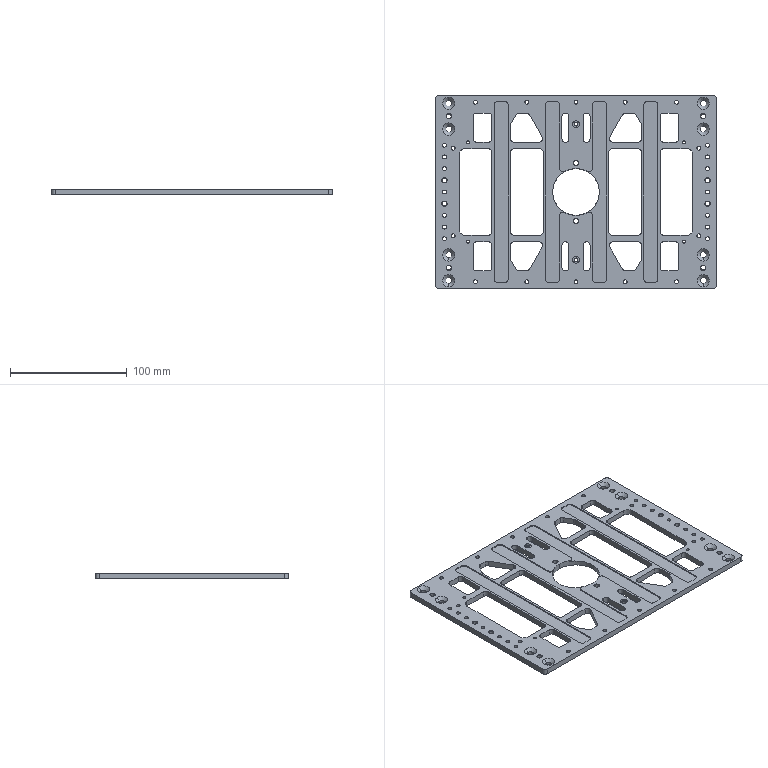NC program | NX | posted with a generic post | part box 240 x 165 x 5 mm
Lines 1 to 1758 of 12487:
N10 G17 G21 G94 G90
(DRILLING , TOOL : D6A45)
N12 T01 M6
N14 G54
N16 G17 G0 G90 X-42. Y-76.8 S5000 M3
N18 G43 Z30. H1
N20 G94 G81 G98 Z-1. F350. R3.
N22 X-86.
N24 X-108.75 Y-75.75
N26 Y-64.75
N28 Y-53.75
N30 X-92.502 Y-42.502
N32 X-105. Y-37.5
N34 X-112.5 Y-40.
N36 Y-30.
N38 Y-20.
N40 Y-10.
N42 Y0.
N44 Y10.
N46 Y20.
N48 Y30.
N50 Y40.
N52 X-105. Y37.5
N54 X-92.502 Y42.5
N56 X-108.75 Y53.75
N58 Y64.75
N60 Y75.75
N62 X-86. Y76.8
N64 X-42.
N66 X0.
N68 Y58.
N70 Y25.
N72 Y0.
N74 Y-25.
N76 Y-58.
N78 Y-76.8
N80 X42.
N82 X86.
N84 X108.75 Y-75.75
N86 Y-64.75
N88 Y-53.75
N90 X92.5 Y-42.502
N92 X105. Y-37.5
N94 X112.5 Y-40.
N96 Y-30.
N98 Y-20.
N100 Y-10.
N102 Y0.
N104 Y10.
N106 Y20.
N108 Y30.
N110 Y40.
N112 X105. Y37.5
N114 X92.5 Y42.5
N116 X108.75 Y53.75
N118 Y64.75
N120 Y75.75
N122 X86. Y76.8
N124 X42.
N126 G80
N128 G0 X42. Y76.8 Z30.
N130 M5
(DRILLING_COPY , TOOL : 3.3ZT)
N132 T03 M6
N134 G54
N136 G17 G0 G90 X-42. Y76.8 S2000 M3
N138 G43 Z30. H3
N140 G94 G83 G98 Z-7.491 F200. Q2. R3.
N142 X0.
N144 X42.
N146 X86.
N148 X105. Y37.5
N150 X112.5 Y40.
N152 Y30.
N154 Y20.
N156 Y0.
N158 Y-20.
N160 Y-30.
N162 Y-40.
N164 X105. Y-37.5
N166 X86. Y-76.8
N168 X42.
N170 X0.
N172 X-42.
N174 X-86.
N176 X-105. Y-37.5
N178 X-112.5 Y-40.
N180 Y-30.
N182 Y-20.
N184 Y0.
N186 Y20.
N188 Y30.
N190 Y40.
N192 X-105. Y37.5
N194 X-86. Y76.8
N196 G80
N198 G0 X-86. Y76.8 Z30.
N200 M5
(DRILLING_COPY_COPY_1 , TOOL : 3.2ZT)
N202 T16 M6
N204 G54
N206 G17 G0 G90 X0. Y58. S2000 M3
N208 G43 Z30. H16
N210 G94 G83 G98 Z-6.961 F200. Q2. R3.
N212 Y-58.
N214 G80
N216 G0 X0. Y-58. Z30.
N218 M5
(DRILLING_COPY_COPY , TOOL : 2.5ZT)
N220 T02 M6
N222 G54
N224 G17 G0 G90 X-92.502 Y42.5 S2000 M3
N226 G43 Z30. H2
N228 G94 G83 G98 Z-7.251 F150. Q2. R3.
N230 Y-42.502
N232 X92.5
N234 Y42.5
N236 G80
N238 G0 X92.5 Y42.5 Z30.
N240 M5
(DRILLING_COPY_COPY_1_COPY , TOOL : 3.8ZT)
N242 T18 M6
N244 G54
N246 G17 G0 G90 X-108.75 Y64.75 S2000 M3
N248 G43 Z30. H18
N250 G94 G83 G98 Z-7.142 F200. Q2. R3.
N252 X-112.5 Y10.
N254 Y-10.
N256 X-108.75 Y-64.75
N258 X0. Y-25.
N260 Y25.
N262 X108.75 Y64.75
N264 X112.5 Y10.
N266 Y-10.
N268 X108.75 Y-64.75
N270 G80
N272 G0 X108.75 Y-64.75 Z30.
N274 M5
(DRILLING_COPY_COPY_1_COPY_COPY , TOOL : 5.3ZT)
N276 T09 M6
N278 G54
N280 G17 G0 G90 X-108.75 Y-75.75 S2000 M3
N282 G43 Z30. H9
N284 G94 G83 G98 Z-7.592 F200. Q2. R3.
N286 Y-53.75
N288 Y53.75
N290 Y75.75
N292 X108.75
N294 Y53.75
N296 Y-53.75
N298 Y-75.75
N300 G80
N302 G0 X108.75 Y-75.75 Z30.
N304 M5
(ZLEVEL_PROFILE , TOOL : D10)
N306 T15 M6
N308 G54
N310 G17 G0 G90 X-45.413 Y87.6 S9500 M3
N312 G43 Z30. H15
N314 Z1.5
N316 G94 G1 X0. Z-0.88 F1000.
N318 X117. F3000.
N320 G2 X125.1 Y79.5 R8.1
N322 G1 Y-79.5
N324 G2 X117. Y-87.6 R8.1
N326 G1 X-117.
N328 G2 X-125.1 Y-79.5 R8.1
N330 G1 Y79.5
N332 G2 X-117. Y87.6 R8.1
N334 G1 X0.
N336 X117. Z-1.003
N338 X117.636 Y87.575 Z-1.004
N340 X118.267 Y87.5
N342 X118.891 Y87.376 Z-1.005
N344 X119.503 Y87.204 Z-1.006
N346 X120.1 Y86.983
N348 X120.677 Y86.717 Z-1.007
N350 X121.232 Y86.406 Z-1.008
N352 X121.761 Y86.053
N354 X122.261 Y85.659 Z-1.009
N356 X122.728 Y85.228 Z-1.01
N358 X123.159 Y84.761
N360 X123.553 Y84.261 Z-1.011
N362 X123.906 Y83.732 Z-1.012
N364 X124.217 Y83.177
N366 X124.483 Y82.6 Z-1.013
N368 X124.704 Y82.003 Z-1.014
N370 X124.876 Y81.391
N372 X125. Y80.767 Z-1.015
N374 X125.075 Y80.136 Z-1.016
N376 X125.1 Y79.5
N378 Y-79.5 Z-1.184
N380 X125.075 Y-80.136
N382 X125. Y-80.767 Z-1.185
N384 X124.876 Y-81.391 Z-1.186
N386 X124.704 Y-82.003
N388 X124.483 Y-82.6 Z-1.187
N390 X124.217 Y-83.177 Z-1.188
N392 X123.906 Y-83.732
N394 X123.553 Y-84.261 Z-1.189
N396 X123.159 Y-84.761 Z-1.19
N398 X122.728 Y-85.228
N400 X122.261 Y-85.659 Z-1.191
N402 X121.761 Y-86.053 Z-1.192
N404 X121.232 Y-86.406
N406 X120.677 Y-86.717 Z-1.193
N408 X120.1 Y-86.983 Z-1.194
N410 X119.503 Y-87.204
N412 X118.891 Y-87.376 Z-1.195
N414 X118.267 Y-87.5 Z-1.196
N416 X117.636 Y-87.575
N418 X117. Y-87.6 Z-1.197
N420 X-117. Z-1.443
N422 X-117.636 Y-87.575 Z-1.444
N424 X-118.267 Y-87.5
N426 X-118.891 Y-87.376 Z-1.445
N428 X-119.503 Y-87.204 Z-1.446
N430 X-120.1 Y-86.983
N432 X-120.677 Y-86.717 Z-1.447
N434 X-121.232 Y-86.406 Z-1.448
N436 X-121.761 Y-86.053
N438 X-122.261 Y-85.659 Z-1.449
N440 X-122.728 Y-85.228 Z-1.45
N442 X-123.159 Y-84.761
N444 X-123.553 Y-84.261 Z-1.451
N446 X-123.906 Y-83.732 Z-1.452
N448 X-124.217 Y-83.177
N450 X-124.483 Y-82.6 Z-1.453
N452 X-124.704 Y-82.003 Z-1.454
N454 X-124.876 Y-81.391
N456 X-125. Y-80.767 Z-1.455
N458 X-125.075 Y-80.136 Z-1.456
N460 X-125.1 Y-79.5
N462 Y79.5 Z-1.624
N464 X-125.075 Y80.136
N466 X-125. Y80.767 Z-1.625
N468 X-124.876 Y81.391 Z-1.626
N470 X-124.704 Y82.003
N472 X-124.483 Y82.6 Z-1.627
N474 X-124.217 Y83.177 Z-1.628
N476 X-123.906 Y83.732
N478 X-123.553 Y84.261 Z-1.629
N480 X-123.159 Y84.761 Z-1.63
N482 X-122.728 Y85.228
N484 X-122.261 Y85.659 Z-1.631
N486 X-121.761 Y86.053 Z-1.632
N488 X-121.232 Y86.406
N490 X-120.677 Y86.717 Z-1.633
N492 X-120.1 Y86.983 Z-1.634
N494 X-119.503 Y87.204
N496 X-118.891 Y87.376 Z-1.635
N498 X-118.267 Y87.5 Z-1.636
N500 X-117.636 Y87.575
N502 X-117. Y87.6 Z-1.637
N504 X0. Z-1.76
N506 X117. Z-1.883
N508 X117.636 Y87.575 Z-1.884
N510 X118.267 Y87.5
N512 X118.891 Y87.376 Z-1.885
N514 X119.503 Y87.204 Z-1.886
N516 X120.1 Y86.983
N518 X120.677 Y86.717 Z-1.887
N520 X121.232 Y86.406 Z-1.888
N522 X121.761 Y86.053
N524 X122.261 Y85.659 Z-1.889
N526 X122.728 Y85.228 Z-1.89
N528 X123.159 Y84.761
N530 X123.553 Y84.261 Z-1.891
N532 X123.906 Y83.732 Z-1.892
N534 X124.217 Y83.177
N536 X124.483 Y82.6 Z-1.893
N538 X124.704 Y82.003 Z-1.894
N540 X124.876 Y81.391
N542 X125. Y80.767 Z-1.895
N544 X125.075 Y80.136 Z-1.896
N546 X125.1 Y79.5
N548 Y-79.5 Z-2.064
N550 X125.075 Y-80.136
N552 X125. Y-80.767 Z-2.065
N554 X124.876 Y-81.391 Z-2.066
N556 X124.704 Y-82.003
N558 X124.483 Y-82.6 Z-2.067
N560 X124.217 Y-83.177 Z-2.068
N562 X123.906 Y-83.732
N564 X123.553 Y-84.261 Z-2.069
N566 X123.159 Y-84.761 Z-2.07
N568 X122.728 Y-85.228
N570 X122.261 Y-85.659 Z-2.071
N572 X121.761 Y-86.053 Z-2.072
N574 X121.232 Y-86.406
N576 X120.677 Y-86.717 Z-2.073
N578 X120.1 Y-86.983 Z-2.074
N580 X119.503 Y-87.204
N582 X118.891 Y-87.376 Z-2.075
N584 X118.267 Y-87.5 Z-2.076
N586 X117.636 Y-87.575
N588 X117. Y-87.6 Z-2.077
N590 X-117. Z-2.323
N592 X-117.636 Y-87.575 Z-2.324
N594 X-118.267 Y-87.5
N596 X-118.891 Y-87.376 Z-2.325
N598 X-119.503 Y-87.204 Z-2.326
N600 X-120.1 Y-86.983
N602 X-120.677 Y-86.717 Z-2.327
N604 X-121.232 Y-86.406 Z-2.328
N606 X-121.761 Y-86.053
N608 X-122.261 Y-85.659 Z-2.329
N610 X-122.728 Y-85.228 Z-2.33
N612 X-123.159 Y-84.761
N614 X-123.553 Y-84.261 Z-2.331
N616 X-123.906 Y-83.732 Z-2.332
N618 X-124.217 Y-83.177
N620 X-124.483 Y-82.6 Z-2.333
N622 X-124.704 Y-82.003 Z-2.334
N624 X-124.876 Y-81.391
N626 X-125. Y-80.767 Z-2.335
N628 X-125.075 Y-80.136 Z-2.336
N630 X-125.1 Y-79.5
N632 Y79.5 Z-2.504
N634 X-125.075 Y80.136
N636 X-125. Y80.767 Z-2.505
N638 X-124.876 Y81.391 Z-2.506
N640 X-124.704 Y82.003
N642 X-124.483 Y82.6 Z-2.507
N644 X-124.217 Y83.177 Z-2.508
N646 X-123.906 Y83.732
N648 X-123.553 Y84.261 Z-2.509
N650 X-123.159 Y84.761 Z-2.51
N652 X-122.728 Y85.228
N654 X-122.261 Y85.659 Z-2.511
N656 X-121.761 Y86.053 Z-2.512
N658 X-121.232 Y86.406
N660 X-120.677 Y86.717 Z-2.513
N662 X-120.1 Y86.983 Z-2.514
N664 X-119.503 Y87.204
N666 X-118.891 Y87.376 Z-2.515
N668 X-118.267 Y87.5 Z-2.516
N670 X-117.636 Y87.575
N672 X-117. Y87.6 Z-2.517
N674 X0. Z-2.64
N676 X117. Z-2.763
N678 X117.636 Y87.575 Z-2.764
N680 X118.267 Y87.5
N682 X118.891 Y87.376 Z-2.765
N684 X119.503 Y87.204 Z-2.766
N686 X120.1 Y86.983
N688 X120.677 Y86.717 Z-2.767
N690 X121.232 Y86.406 Z-2.768
N692 X121.761 Y86.053
N694 X122.261 Y85.659 Z-2.769
N696 X122.728 Y85.228 Z-2.77
N698 X123.159 Y84.761
N700 X123.553 Y84.261 Z-2.771
N702 X123.906 Y83.732 Z-2.772
N704 X124.217 Y83.177
N706 X124.483 Y82.6 Z-2.773
N708 X124.704 Y82.003 Z-2.774
N710 X124.876 Y81.391
N712 X125. Y80.767 Z-2.775
N714 X125.075 Y80.136 Z-2.776
N716 X125.1 Y79.5
N718 Y-79.5 Z-2.944
N720 X125.075 Y-80.136
N722 X125. Y-80.767 Z-2.945
N724 X124.876 Y-81.391 Z-2.946
N726 X124.704 Y-82.003
N728 X124.483 Y-82.6 Z-2.947
N730 X124.217 Y-83.177 Z-2.948
N732 X123.906 Y-83.732
N734 X123.553 Y-84.261 Z-2.949
N736 X123.159 Y-84.761 Z-2.95
N738 X122.728 Y-85.228
N740 X122.261 Y-85.659 Z-2.951
N742 X121.761 Y-86.053 Z-2.952
N744 X121.232 Y-86.406
N746 X120.677 Y-86.717 Z-2.953
N748 X120.1 Y-86.983 Z-2.954
N750 X119.503 Y-87.204
N752 X118.891 Y-87.376 Z-2.955
N754 X118.267 Y-87.5 Z-2.956
N756 X117.636 Y-87.575
N758 X117. Y-87.6 Z-2.957
N760 X-117. Z-3.203
N762 X-117.636 Y-87.575 Z-3.204
N764 X-118.267 Y-87.5
N766 X-118.891 Y-87.376 Z-3.205
N768 X-119.503 Y-87.204 Z-3.206
N770 X-120.1 Y-86.983
N772 X-120.677 Y-86.717 Z-3.207
N774 X-121.232 Y-86.406 Z-3.208
N776 X-121.761 Y-86.053
N778 X-122.261 Y-85.659 Z-3.209
N780 X-122.728 Y-85.228 Z-3.21
N782 X-123.159 Y-84.761
N784 X-123.553 Y-84.261 Z-3.211
N786 X-123.906 Y-83.732 Z-3.212
N788 X-124.217 Y-83.177
N790 X-124.483 Y-82.6 Z-3.213
N792 X-124.704 Y-82.003 Z-3.214
N794 X-124.876 Y-81.391
N796 X-125. Y-80.767 Z-3.215
N798 X-125.075 Y-80.136 Z-3.216
N800 X-125.1 Y-79.5
N802 Y79.5 Z-3.384
N804 X-125.075 Y80.136
N806 X-125. Y80.767 Z-3.385
N808 X-124.876 Y81.391 Z-3.386
N810 X-124.704 Y82.003
N812 X-124.483 Y82.6 Z-3.387
N814 X-124.217 Y83.177 Z-3.388
N816 X-123.906 Y83.732
N818 X-123.553 Y84.261 Z-3.389
N820 X-123.159 Y84.761 Z-3.39
N822 X-122.728 Y85.228
N824 X-122.261 Y85.659 Z-3.391
N826 X-121.761 Y86.053 Z-3.392
N828 X-121.232 Y86.406
N830 X-120.677 Y86.717 Z-3.393
N832 X-120.1 Y86.983 Z-3.394
N834 X-119.503 Y87.204
N836 X-118.891 Y87.376 Z-3.395
N838 X-118.267 Y87.5 Z-3.396
N840 X-117.636 Y87.575
N842 X-117. Y87.6 Z-3.397
N844 X0. Z-3.52
N846 X117. Z-3.643
N848 X117.636 Y87.575 Z-3.644
N850 X118.267 Y87.5
N852 X118.891 Y87.376 Z-3.645
N854 X119.503 Y87.204 Z-3.646
N856 X120.1 Y86.983
N858 X120.677 Y86.717 Z-3.647
N860 X121.232 Y86.406 Z-3.648
N862 X121.761 Y86.053
N864 X122.261 Y85.659 Z-3.649
N866 X122.728 Y85.228 Z-3.65
N868 X123.159 Y84.761
N870 X123.553 Y84.261 Z-3.651
N872 X123.906 Y83.732 Z-3.652
N874 X124.217 Y83.177
N876 X124.483 Y82.6 Z-3.653
N878 X124.704 Y82.003 Z-3.654
N880 X124.876 Y81.391
N882 X125. Y80.767 Z-3.655
N884 X125.075 Y80.136 Z-3.656
N886 X125.1 Y79.5
N888 Y-79.5 Z-3.824
N890 X125.075 Y-80.136
N892 X125. Y-80.767 Z-3.825
N894 X124.876 Y-81.391 Z-3.826
N896 X124.704 Y-82.003
N898 X124.483 Y-82.6 Z-3.827
N900 X124.217 Y-83.177 Z-3.828
N902 X123.906 Y-83.732
N904 X123.553 Y-84.261 Z-3.829
N906 X123.159 Y-84.761 Z-3.83
N908 X122.728 Y-85.228
N910 X122.261 Y-85.659 Z-3.831
N912 X121.761 Y-86.053 Z-3.832
N914 X121.232 Y-86.406
N916 X120.677 Y-86.717 Z-3.833
N918 X120.1 Y-86.983 Z-3.834
N920 X119.503 Y-87.204
N922 X118.891 Y-87.376 Z-3.835
N924 X118.267 Y-87.5 Z-3.836
N926 X117.636 Y-87.575
N928 X117. Y-87.6 Z-3.837
N930 X-117. Z-4.083
N932 X-117.636 Y-87.575 Z-4.084
N934 X-118.267 Y-87.5
N936 X-118.891 Y-87.376 Z-4.085
N938 X-119.503 Y-87.204 Z-4.086
N940 X-120.1 Y-86.983
N942 X-120.677 Y-86.717 Z-4.087
N944 X-121.232 Y-86.406 Z-4.088
N946 X-121.761 Y-86.053
N948 X-122.261 Y-85.659 Z-4.089
N950 X-122.728 Y-85.228 Z-4.09
N952 X-123.159 Y-84.761
N954 X-123.553 Y-84.261 Z-4.091
N956 X-123.906 Y-83.732 Z-4.092
N958 X-124.217 Y-83.177
N960 X-124.483 Y-82.6 Z-4.093
N962 X-124.704 Y-82.003 Z-4.094
N964 X-124.876 Y-81.391
N966 X-125. Y-80.767 Z-4.095
N968 X-125.075 Y-80.136 Z-4.096
N970 X-125.1 Y-79.5
N972 Y79.5 Z-4.264
N974 X-125.075 Y80.136
N976 X-125. Y80.767 Z-4.265
N978 X-124.876 Y81.391 Z-4.266
N980 X-124.704 Y82.003
N982 X-124.483 Y82.6 Z-4.267
N984 X-124.217 Y83.177 Z-4.268
N986 X-123.906 Y83.732
N988 X-123.553 Y84.261 Z-4.269
N990 X-123.159 Y84.761 Z-4.27
N992 X-122.728 Y85.228
N994 X-122.261 Y85.659 Z-4.271
N996 X-121.761 Y86.053 Z-4.272
N998 X-121.232 Y86.406
N1000 X-120.677 Y86.717 Z-4.273
N1002 X-120.1 Y86.983 Z-4.274
N1004 X-119.503 Y87.204
N1006 X-118.891 Y87.376 Z-4.275
N1008 X-118.267 Y87.5 Z-4.276
N1010 X-117.636 Y87.575
N1012 X-117. Y87.6 Z-4.277
N1014 X0. Z-4.4
N1016 X117.
N1018 G2 X125.1 Y79.5 R8.1
N1020 G1 Y-79.5
N1022 G2 X117. Y-87.6 R8.1
N1024 G1 X-117.
N1026 G2 X-125.1 Y-79.5 R8.1
N1028 G1 Y79.5
N1030 G2 X-117. Y87.6 R8.1
N1032 G1 X0.
N1034 Z-2.9
N1036 G0 Z30.
(ZLEVEL_PROFILE_COPY , TOOL : D10)
N1038 X77.1 Y61.503
N1040 Z1.5
N1042 G1 Y47.6 Z0.771 F1000.
N1044 X82.9 Z0.467
N1046 Y62.4 Z-0.308
N1048 X77.1 Z-0.612
N1050 Y55. Z-1.
N1052 Y47.6 F3000.
N1054 X82.9
N1056 Y62.4
N1058 X77.1
N1060 Y55.
N1062 Y47.6 Z-1.18
N1064 X82.9 Z-1.32
N1066 Y62.4 Z-1.68
N1068 X77.1 Z-1.82
N1070 Y55. Z-2.
N1072 Y47.6 Z-2.18
N1074 X82.9 Z-2.32
N1076 Y62.4 Z-2.68
N1078 X77.1 Z-2.82
N1080 Y55. Z-3.
N1082 Y47.6 Z-3.18
N1084 X82.9 Z-3.32
N1086 Y62.4 Z-3.68
N1088 X77.1 Z-3.82
N1090 Y55. Z-4.
N1092 Y47.6 Z-4.18
N1094 X82.9 Z-4.32
N1096 Y62.4 Z-4.68
N1098 X77.1 Z-4.82
N1100 Y55. Z-5.
N1102 Y47.6
N1104 X82.9
N1106 Y62.4
N1108 X77.1
N1110 Y55.
N1112 Z-3.5
N1114 G0 Z53.
N1116 X-41.675 Y58.887
N1118 Z1.5
N1120 G1 X-43.703 Y62.4 Z1.287 F1000.
N1122 X-47.297 Z1.099
N1124 X-50.9 Y56.16 Z0.721
N1126 Y47.6 Z0.273
N1128 X-35.158 Z-0.552
N1130 X-39.43 Y55. Z-1.
N1132 X-43.703 Y62.4 F3000.
N1134 X-47.297
N1136 X-50.9 Y56.16
N1138 Y47.6
N1140 X-35.158
N1142 X-39.43 Y55.
N1144 X-43.703 Y62.4 Z-1.164
N1146 X-47.297 Z-1.233
N1148 X-50.9 Y56.16 Z-1.371
N1150 Y47.6 Z-1.535
N1152 X-35.158 Z-1.836
N1154 X-39.43 Y55. Z-2.
N1156 X-43.703 Y62.4 Z-2.164
N1158 X-47.297 Z-2.233
N1160 X-50.9 Y56.16 Z-2.371
N1162 Y47.6 Z-2.535
N1164 X-35.158 Z-2.836
N1166 X-39.43 Y55. Z-3.
N1168 X-43.703 Y62.4 Z-3.164
N1170 X-47.297 Z-3.233
N1172 X-50.9 Y56.16 Z-3.371
N1174 Y47.6 Z-3.535
N1176 X-35.158 Z-3.836
N1178 X-39.43 Y55. Z-4.
N1180 X-43.703 Y62.4 Z-4.164
N1182 X-47.297 Z-4.233
N1184 X-50.9 Y56.16 Z-4.371
N1186 Y47.6 Z-4.535
N1188 X-35.158 Z-4.836
N1190 X-39.43 Y55. Z-5.
N1192 X-43.703 Y62.4
N1194 X-47.297
N1196 X-50.9 Y56.16
N1198 Y47.6
N1200 X-35.158
N1202 X-39.43 Y55.
N1204 Z-3.5
N1206 G0 Z53.
N1208 X77.1 Y-48.497
N1210 Z1.5
N1212 G1 Y-62.4 Z0.771 F1000.
N1214 X82.9 Z0.467
N1216 Y-47.6 Z-0.308
N1218 X77.1 Z-0.612
N1220 Y-55. Z-1.
N1222 Y-62.4 F3000.
N1224 X82.9
N1226 Y-47.6
N1228 X77.1
N1230 Y-55.
N1232 Y-62.4 Z-1.18
N1234 X82.9 Z-1.32
N1236 Y-47.6 Z-1.68
N1238 X77.1 Z-1.82
N1240 Y-55. Z-2.
N1242 Y-62.4 Z-2.18
N1244 X82.9 Z-2.32
N1246 Y-47.6 Z-2.68
N1248 X77.1 Z-2.82
N1250 Y-55. Z-3.
N1252 Y-62.4 Z-3.18
N1254 X82.9 Z-3.32
N1256 Y-47.6 Z-3.68
N1258 X77.1 Z-3.82
N1260 Y-55. Z-4.
N1262 Y-62.4 Z-4.18
N1264 X82.9 Z-4.32
N1266 Y-47.6 Z-4.68
N1268 X77.1 Z-4.82
N1270 Y-55. Z-5.
N1272 Y-62.4
N1274 X82.9
N1276 Y-47.6
N1278 X77.1
N1280 Y-55.
N1282 Z-3.5
N1284 G0 Z53.
N1286 X50.9 Y-50.994
N1288 Z1.5
N1290 G1 Y-47.6 Z1.322 F1000.
N1292 X35.158 Z0.497
N1294 X43.703 Y-62.4 Z-0.399
N1296 X47.297 Z-0.587
N1298 X50.9 Y-56.16 Z-0.965
N1300 Y-55.483 Z-1.
N1302 Y-47.6 F3000.
N1304 X35.158
N1306 X43.703 Y-62.4
N1308 X47.297
N1310 X50.9 Y-56.16
N1312 Y-55.483
N1314 Y-47.6 Z-1.151
N1316 X35.158 Z-1.453
N1318 X43.703 Y-62.4 Z-1.78
N1320 X47.297 Z-1.849
N1322 X50.9 Y-56.16 Z-1.987
N1324 Y-55.483 Z-2.
N1326 Y-47.6 Z-2.151
N1328 X35.158 Z-2.453
N1330 X43.703 Y-62.4 Z-2.78
N1332 X47.297 Z-2.849
N1334 X50.9 Y-56.16 Z-2.987
N1336 Y-55.483 Z-3.
N1338 Y-47.6 Z-3.151
N1340 X35.158 Z-3.453
N1342 X43.703 Y-62.4 Z-3.78
N1344 X47.297 Z-3.849
N1346 X50.9 Y-56.16 Z-3.987
N1348 Y-55.483 Z-4.
N1350 Y-47.6 Z-4.151
N1352 X35.158 Z-4.453
N1354 X43.703 Y-62.4 Z-4.78
N1356 X47.297 Z-4.849
N1358 X50.9 Y-56.16 Z-4.987
N1360 Y-55.483 Z-5.
N1362 Y-47.6
N1364 X35.158
N1366 X43.703 Y-62.4
N1368 X47.297
N1370 X50.9 Y-56.16
N1372 Y-55.483
N1374 Z-3.5
N1376 G0 Z53.
N1378 X-37.186 Y-51.113
N1380 Z1.5
N1382 G1 X-35.158 Y-47.6 Z1.287 F1000.
N1384 X-50.9 Z0.462
N1386 Y-56.16 Z0.014
N1388 X-47.297 Y-62.4 Z-0.364
N1390 X-43.703 Z-0.552
N1392 X-39.43 Y-55. Z-1.
N1394 X-35.158 Y-47.6 F3000.
N1396 X-50.9
N1398 Y-56.16
N1400 X-47.297 Y-62.4
N1402 X-43.703
N1404 X-39.43 Y-55.
N1406 X-35.158 Y-47.6 Z-1.164
N1408 X-50.9 Z-1.465
N1410 Y-56.16 Z-1.629
N1412 X-47.297 Y-62.4 Z-1.767
N1414 X-43.703 Z-1.836
N1416 X-39.43 Y-55. Z-2.
N1418 X-35.158 Y-47.6 Z-2.164
N1420 X-50.9 Z-2.465
N1422 Y-56.16 Z-2.629
N1424 X-47.297 Y-62.4 Z-2.767
N1426 X-43.703 Z-2.836
N1428 X-39.43 Y-55. Z-3.
N1430 X-35.158 Y-47.6 Z-3.164
N1432 X-50.9 Z-3.465
N1434 Y-56.16 Z-3.629
N1436 X-47.297 Y-62.4 Z-3.767
N1438 X-43.703 Z-3.836
N1440 X-39.43 Y-55. Z-4.
N1442 X-35.158 Y-47.6 Z-4.164
N1444 X-50.9 Z-4.465
N1446 Y-56.16 Z-4.629
N1448 X-47.297 Y-62.4 Z-4.767
N1450 X-43.703 Z-4.836
N1452 X-39.43 Y-55. Z-5.
N1454 X-35.158 Y-47.6
N1456 X-50.9
N1458 Y-56.16
N1460 X-47.297 Y-62.4
N1462 X-43.703
N1464 X-39.43 Y-55.
N1466 Z-3.5
N1468 G0 Z53.
N1470 X37.186 Y51.113
N1472 Z1.5
N1474 G1 X35.158 Y47.6 Z1.287 F1000.
N1476 X50.9 Z0.462
N1478 Y56.16 Z0.014
N1480 X47.297 Y62.4 Z-0.364
N1482 X43.703 Z-0.552
N1484 X39.43 Y55. Z-1.
N1486 X35.158 Y47.6 F3000.
N1488 X50.9
N1490 Y56.16
N1492 X47.297 Y62.4
N1494 X43.703
N1496 X39.43 Y55.
N1498 X35.158 Y47.6 Z-1.164
N1500 X50.9 Z-1.465
N1502 Y56.16 Z-1.629
N1504 X47.297 Y62.4 Z-1.767
N1506 X43.703 Z-1.836
N1508 X39.43 Y55. Z-2.
N1510 X35.158 Y47.6 Z-2.164
N1512 X50.9 Z-2.465
N1514 Y56.16 Z-2.629
N1516 X47.297 Y62.4 Z-2.767
N1518 X43.703 Z-2.836
N1520 X39.43 Y55. Z-3.
N1522 X35.158 Y47.6 Z-3.164
N1524 X50.9 Z-3.465
N1526 Y56.16 Z-3.629
N1528 X47.297 Y62.4 Z-3.767
N1530 X43.703 Z-3.836
N1532 X39.43 Y55. Z-4.
N1534 X35.158 Y47.6 Z-4.164
N1536 X50.9 Z-4.465
N1538 Y56.16 Z-4.629
N1540 X47.297 Y62.4 Z-4.767
N1542 X43.703 Z-4.836
N1544 X39.43 Y55. Z-5.
N1546 X35.158 Y47.6
N1548 X50.9
N1550 Y56.16
N1552 X47.297 Y62.4
N1554 X43.703
N1556 X39.43 Y55.
N1558 Z-3.5
N1560 G0 Z53.
N1562 X-77.1 Y-61.503
N1564 Z1.5
N1566 G1 Y-47.6 Z0.771 F1000.
N1568 X-82.9 Z0.467
N1570 Y-62.4 Z-0.308
N1572 X-77.1 Z-0.612
N1574 Y-55. Z-1.
N1576 Y-47.6 F3000.
N1578 X-82.9
N1580 Y-62.4
N1582 X-77.1
N1584 Y-55.
N1586 Y-47.6 Z-1.18
N1588 X-82.9 Z-1.32
N1590 Y-62.4 Z-1.68
N1592 X-77.1 Z-1.82
N1594 Y-55. Z-2.
N1596 Y-47.6 Z-2.18
N1598 X-82.9 Z-2.32
N1600 Y-62.4 Z-2.68
N1602 X-77.1 Z-2.82
N1604 Y-55. Z-3.
N1606 Y-47.6 Z-3.18
N1608 X-82.9 Z-3.32
N1610 Y-62.4 Z-3.68
N1612 X-77.1 Z-3.82
N1614 Y-55. Z-4.
N1616 Y-47.6 Z-4.18
N1618 X-82.9 Z-4.32
N1620 Y-62.4 Z-4.68
N1622 X-77.1 Z-4.82
N1624 Y-55. Z-5.
N1626 Y-47.6
N1628 X-82.9
N1630 Y-62.4
N1632 X-77.1
N1634 Y-55.
N1636 Z-3.5
N1638 G0 Z53.
N1640 Y48.497
N1642 Z1.5
N1644 G1 Y62.4 Z0.771 F1000.
N1646 X-82.9 Z0.467
N1648 Y47.6 Z-0.308
N1650 X-77.1 Z-0.612
N1652 Y55. Z-1.
N1654 Y62.4 F3000.
N1656 X-82.9
N1658 Y47.6
N1660 X-77.1
N1662 Y55.
N1664 Y62.4 Z-1.18
N1666 X-82.9 Z-1.32
N1668 Y47.6 Z-1.68
N1670 X-77.1 Z-1.82
N1672 Y55. Z-2.
N1674 Y62.4 Z-2.18
N1676 X-82.9 Z-2.32
N1678 Y47.6 Z-2.68
N1680 X-77.1 Z-2.82
N1682 Y55. Z-3.
N1684 Y62.4 Z-3.18
N1686 X-82.9 Z-3.32
N1688 Y47.6 Z-3.68
N1690 X-77.1 Z-3.82
N1692 Y55. Z-4.
N1694 Y62.4 Z-4.18
N1696 X-82.9 Z-4.32
N1698 Y47.6 Z-4.68
N1700 X-77.1 Z-4.82
N1702 Y55. Z-5.
N1704 Y62.4
N1706 X-82.9
N1708 Y47.6
N1710 X-77.1
N1712 Y55.
N1714 Z-3.5
N1716 G0 Z30.
(PLANAR_MILL , TOOL : D10)
N1718 X-84.1 Y5.897
N1720 Z1.5
N1722 G1 Y24.9 Z0.504
N1724 X-87.9 Z0.305
N1726 Y0. Z-1.
N1728 Y-24.9
N1730 X-84.1
N1732 Y24.9
N1734 X-87.9
N1736 Y0.
N1738 X-94.9
N1740 Y-31.9
N1742 X-77.1
N1744 Y31.9
N1746 X-94.9
N1748 Y0.
N1750 Z0.5
N1752 G0 X-84.1 Y5.897
N1754 G1 Y24.9 Z-0.496
N1756 X-87.9 Z-0.695
N1758 Y0. Z-2.
N1760 Y-24.9
N1762 X-84.1
N1764 Y24.9
N1766 X-87.9
N1768 Y0.
N1770 X-94.9
N1772 Y-31.9
N1774 X-77.1
N1776 Y31.9
N1778 X-94.9
N1780 Y0.
N1782 Z-0.5
N1784 G0 X-84.1 Y5.897
N1786 G1 Y24.9 Z-1.496
N1788 X-87.9 Z-1.695
N1790 Y0. Z-3.
N1792 Y-24.9
N1794 X-84.1
N1796 Y24.9
N1798 X-87.9
N1800 Y0.
N1802 X-94.9
N1804 Y-31.9
N1806 X-77.1
N1808 Y31.9
N1810 X-94.9
N1812 Y0.
N1814 Z-1.5
N1816 G0 X-84.1 Y5.897
N1818 G1 Y24.9 Z-2.496
N1820 X-87.9 Z-2.695
N1822 Y0. Z-4.
N1824 Y-24.9
N1826 X-84.1
N1828 Y24.9
N1830 X-87.9
N1832 Y0.
N1834 X-94.9
N1836 Y-31.9
N1838 X-77.1
N1840 Y31.9
N1842 X-94.9
N1844 Y0.
N1846 Z-2.5
N1848 G0 X-84.1 Y5.897
N1850 G1 Y24.9 Z-3.496
N1852 X-87.9 Z-3.695
N1854 Y0. Z-5.
N1856 Y-24.9
N1858 X-84.1
N1860 Y24.9
N1862 X-87.9
N1864 Y0.
N1866 X-94.9
N1868 Y-31.9
N1870 X-77.1
N1872 Y31.9
N1874 X-94.9
N1876 Y0.
N1878 Z-3.5
N1880 G0 Z30.
N1882 X-40.1 Y5.897
N1884 Z1.5
N1886 G1 Y24.9 Z0.504
N1888 X-43.9 Z0.305
N1890 Y0. Z-1.
N1892 Y-24.9
N1894 X-40.1
N1896 Y24.9
N1898 X-43.9
N1900 Y0.
N1902 X-50.9
N1904 Y-31.9
N1906 X-33.1
N1908 Y31.9
N1910 X-50.9
N1912 Y0.
N1914 Z0.5
N1916 G0 X-40.1 Y5.897
N1918 G1 Y24.9 Z-0.496
N1920 X-43.9 Z-0.695
N1922 Y0. Z-2.
N1924 Y-24.9
N1926 X-40.1
N1928 Y24.9
N1930 X-43.9
N1932 Y0.
N1934 X-50.9
N1936 Y-31.9
N1938 X-33.1
N1940 Y31.9
N1942 X-50.9
N1944 Y0.
N1946 Z-0.5
N1948 G0 X-40.1 Y5.897
N1950 G1 Y24.9 Z-1.496
N1952 X-43.9 Z-1.695
N1954 Y0. Z-3.
N1956 Y-24.9
N1958 X-40.1
N1960 Y24.9
N1962 X-43.9
N1964 Y0.
N1966 X-50.9
N1968 Y-31.9
N1970 X-33.1
N1972 Y31.9
N1974 X-50.9
N1976 Y0.
N1978 Z-1.5
N1980 G0 X-40.1 Y5.897
N1982 G1 Y24.9 Z-2.496
N1984 X-43.9 Z-2.695
N1986 Y0. Z-4.
N1988 Y-24.9
N1990 X-40.1
N1992 Y24.9
N1994 X-43.9
N1996 Y0.
N1998 X-50.9
N2000 Y-31.9
N2002 X-33.1
N2004 Y31.9
N2006 X-50.9
N2008 Y0.
N2010 Z-2.5
N2012 G0 X-40.1 Y5.897
N2014 G1 Y24.9 Z-3.496
N2016 X-43.9 Z-3.695
N2018 Y0. Z-5.
N2020 Y-24.9
N2022 X-40.1
N2024 Y24.9
N2026 X-43.9
N2028 Y0.
N2030 X-50.9
N2032 Y-31.9
N2034 X-33.1
N2036 Y31.9
N2038 X-50.9
N2040 Y0.
N2042 Z-3.5
N2044 G0 Z30.
N2046 X1.989 Y-7.632
N2048 Z1.5
N2050 G1 X2.493 Y-7.528 Z1.473
N2052 X4.162 Y-6.75 Z1.376
N2054 X5.607 Y-5.607 Z1.28
N2056 X6.75 Y-4.162 Z1.183
N2058 X7.528 Y-2.493 Z1.087
N2060 X7.9 Y-0.689 Z0.99
N2062 Y0.689 Z0.918
N2064 X7.528 Y2.493 Z0.822
N2066 X6.75 Y4.162 Z0.725
N2068 X5.607 Y5.607 Z0.629
N2070 X4.162 Y6.75 Z0.532
N2072 X2.493 Y7.528 Z0.435
N2074 X0.689 Y7.9 Z0.339
N2076 X-0.689 Z0.267
N2078 X-2.493 Y7.528 Z0.17
N2080 X-4.162 Y6.75 Z0.074
N2082 X-5.607 Y5.607 Z-0.023
N2084 X-6.75 Y4.162 Z-0.119
N2086 X-7.528 Y2.493 Z-0.216
N2088 X-7.9 Y0.689 Z-0.312
N2090 Y-0.689 Z-0.385
N2092 X-7.528 Y-2.493 Z-0.481
N2094 X-6.75 Y-4.162 Z-0.578
N2096 X-5.607 Y-5.607 Z-0.674
N2098 X-4.162 Y-6.75 Z-0.771
N2100 X-2.493 Y-7.528 Z-0.867
N2102 X-0.689 Y-7.9 Z-0.964
N2104 X0. Z-1.
N2106 Y-0.9
N2108 G3 X0.9 Y0. R0.9
N2110 X0. Y-0.9 R-0.9
N2112 G1 Y-7.9
N2114 G3 X7.9 Y0. R7.9
N2116 X0. Y-7.9 R-7.9
N2118 G1 Y-14.9
N2120 G3 X14.9 Y0. R14.9
N2122 X0. Y-14.9 R-14.9
N2124 G1 Z0.5
N2126 G0 X1.989 Y-7.632
N2128 G1 X2.493 Y-7.528 Z0.473
N2130 X4.162 Y-6.75 Z0.376
N2132 X5.607 Y-5.607 Z0.28
N2134 X6.75 Y-4.162 Z0.183
N2136 X7.528 Y-2.493 Z0.087
N2138 X7.9 Y-0.689 Z-0.01
N2140 Y0.689 Z-0.082
N2142 X7.528 Y2.493 Z-0.178
N2144 X6.75 Y4.162 Z-0.275
N2146 X5.607 Y5.607 Z-0.371
N2148 X4.162 Y6.75 Z-0.468
N2150 X2.493 Y7.528 Z-0.565
N2152 X0.689 Y7.9 Z-0.661
N2154 X-0.689 Z-0.733
N2156 X-2.493 Y7.528 Z-0.83
N2158 X-4.162 Y6.75 Z-0.926
N2160 X-5.607 Y5.607 Z-1.023
N2162 X-6.75 Y4.162 Z-1.119
N2164 X-7.528 Y2.493 Z-1.216
N2166 X-7.9 Y0.689 Z-1.312
N2168 Y-0.689 Z-1.385
N2170 X-7.528 Y-2.493 Z-1.481
N2172 X-6.75 Y-4.162 Z-1.578
N2174 X-5.607 Y-5.607 Z-1.674
N2176 X-4.162 Y-6.75 Z-1.771
N2178 X-2.493 Y-7.528 Z-1.867
N2180 X-0.689 Y-7.9 Z-1.964
N2182 X0. Z-2.
N2184 Y-0.9
N2186 G3 X0.9 Y0. R0.9
N2188 X0. Y-0.9 R-0.9
N2190 G1 Y-7.9
N2192 G3 X7.9 Y0. R7.9
N2194 X0. Y-7.9 R-7.9
N2196 G1 Y-14.9
N2198 G3 X14.9 Y0. R14.9
N2200 X0. Y-14.9 R-14.9
N2202 G1 Z-0.5
N2204 G0 X1.989 Y-7.632
N2206 G1 X2.493 Y-7.528 Z-0.527
N2208 X4.162 Y-6.75 Z-0.624
N2210 X5.607 Y-5.607 Z-0.72
N2212 X6.75 Y-4.162 Z-0.817
N2214 X7.528 Y-2.493 Z-0.913
N2216 X7.9 Y-0.689 Z-1.01
N2218 Y0.689 Z-1.082
N2220 X7.528 Y2.493 Z-1.178
N2222 X6.75 Y4.162 Z-1.275
N2224 X5.607 Y5.607 Z-1.371
N2226 X4.162 Y6.75 Z-1.468
N2228 X2.493 Y7.528 Z-1.565
N2230 X0.689 Y7.9 Z-1.661
N2232 X-0.689 Z-1.733
N2234 X-2.493 Y7.528 Z-1.83
N2236 X-4.162 Y6.75 Z-1.926
N2238 X-5.607 Y5.607 Z-2.023
N2240 X-6.75 Y4.162 Z-2.119
N2242 X-7.528 Y2.493 Z-2.216
N2244 X-7.9 Y0.689 Z-2.312
N2246 Y-0.689 Z-2.385
N2248 X-7.528 Y-2.493 Z-2.481
N2250 X-6.75 Y-4.162 Z-2.578
N2252 X-5.607 Y-5.607 Z-2.674
N2254 X-4.162 Y-6.75 Z-2.771
N2256 X-2.493 Y-7.528 Z-2.867
N2258 X-0.689 Y-7.9 Z-2.964
N2260 X0. Z-3.
N2262 Y-0.9
N2264 G3 X0.9 Y0. R0.9
N2266 X0. Y-0.9 R-0.9
N2268 G1 Y-7.9
N2270 G3 X7.9 Y0. R7.9
N2272 X0. Y-7.9 R-7.9
N2274 G1 Y-14.9
N2276 G3 X14.9 Y0. R14.9
N2278 X0. Y-14.9 R-14.9
N2280 G1 Z-1.5
N2282 G0 X1.989 Y-7.632
N2284 G1 X2.493 Y-7.528 Z-1.527
N2286 X4.162 Y-6.75 Z-1.624
N2288 X5.607 Y-5.607 Z-1.72
N2290 X6.75 Y-4.162 Z-1.817
N2292 X7.528 Y-2.493 Z-1.913
N2294 X7.9 Y-0.689 Z-2.01
N2296 Y0.689 Z-2.082
N2298 X7.528 Y2.493 Z-2.178
N2300 X6.75 Y4.162 Z-2.275
N2302 X5.607 Y5.607 Z-2.371
N2304 X4.162 Y6.75 Z-2.468
N2306 X2.493 Y7.528 Z-2.565
N2308 X0.689 Y7.9 Z-2.661
N2310 X-0.689 Z-2.733
N2312 X-2.493 Y7.528 Z-2.83
N2314 X-4.162 Y6.75 Z-2.926
N2316 X-5.607 Y5.607 Z-3.023
N2318 X-6.75 Y4.162 Z-3.119
N2320 X-7.528 Y2.493 Z-3.216
N2322 X-7.9 Y0.689 Z-3.312
N2324 Y-0.689 Z-3.385
N2326 X-7.528 Y-2.493 Z-3.481
N2328 X-6.75 Y-4.162 Z-3.578
N2330 X-5.607 Y-5.607 Z-3.674
N2332 X-4.162 Y-6.75 Z-3.771
N2334 X-2.493 Y-7.528 Z-3.867
N2336 X-0.689 Y-7.9 Z-3.964
N2338 X0. Z-4.
N2340 Y-0.9
N2342 G3 X0.9 Y0. R0.9
N2344 X0. Y-0.9 R-0.9
N2346 G1 Y-7.9
N2348 G3 X7.9 Y0. R7.9
N2350 X0. Y-7.9 R-7.9
N2352 G1 Y-14.9
N2354 G3 X14.9 Y0. R14.9
N2356 X0. Y-14.9 R-14.9
N2358 G1 Z-2.5
N2360 G0 X1.989 Y-7.632
N2362 G1 X2.493 Y-7.528 Z-2.527
N2364 X4.162 Y-6.75 Z-2.624
N2366 X5.607 Y-5.607 Z-2.72
N2368 X6.75 Y-4.162 Z-2.817
N2370 X7.528 Y-2.493 Z-2.913
N2372 X7.9 Y-0.689 Z-3.01
N2374 Y0.689 Z-3.082
N2376 X7.528 Y2.493 Z-3.178
N2378 X6.75 Y4.162 Z-3.275
N2380 X5.607 Y5.607 Z-3.371
N2382 X4.162 Y6.75 Z-3.468
N2384 X2.493 Y7.528 Z-3.565
N2386 X0.689 Y7.9 Z-3.661
N2388 X-0.689 Z-3.733
N2390 X-2.493 Y7.528 Z-3.83
N2392 X-4.162 Y6.75 Z-3.926
N2394 X-5.607 Y5.607 Z-4.023
N2396 X-6.75 Y4.162 Z-4.119
N2398 X-7.528 Y2.493 Z-4.216
N2400 X-7.9 Y0.689 Z-4.312
N2402 Y-0.689 Z-4.385
N2404 X-7.528 Y-2.493 Z-4.481
N2406 X-6.75 Y-4.162 Z-4.578
N2408 X-5.607 Y-5.607 Z-4.674
N2410 X-4.162 Y-6.75 Z-4.771
N2412 X-2.493 Y-7.528 Z-4.867
N2414 X-0.689 Y-7.9 Z-4.964
N2416 X0. Z-5.
N2418 Y-0.9
N2420 G3 X0.9 Y0. R0.9
N2422 X0. Y-0.9 R-0.9
N2424 G1 Y-7.9
N2426 G3 X7.9 Y0. R7.9
N2428 X0. Y-7.9 R-7.9
N2430 G1 Y-14.9
N2432 G3 X14.9 Y0. R14.9
N2434 X0. Y-14.9 R-14.9
N2436 G1 Z-3.5
N2438 G0 Z30.
N2440 X43.9 Y5.897
N2442 Z1.5
N2444 G1 Y24.9 Z0.504
N2446 X40.1 Z0.305
N2448 Y0. Z-1.
N2450 Y-24.9
N2452 X43.9
N2454 Y24.9
N2456 X40.1
N2458 Y0.
N2460 X33.1
N2462 Y-31.9
N2464 X50.9
N2466 Y31.9
N2468 X33.1
N2470 Y0.
N2472 Z0.5
N2474 G0 X43.9 Y5.897
N2476 G1 Y24.9 Z-0.496
N2478 X40.1 Z-0.695
N2480 Y0. Z-2.
N2482 Y-24.9
N2484 X43.9
N2486 Y24.9
N2488 X40.1
N2490 Y0.
N2492 X33.1
N2494 Y-31.9
N2496 X50.9
N2498 Y31.9
N2500 X33.1
N2502 Y0.
N2504 Z-0.5
N2506 G0 X43.9 Y5.897
N2508 G1 Y24.9 Z-1.496
N2510 X40.1 Z-1.695
N2512 Y0. Z-3.
N2514 Y-24.9
N2516 X43.9
N2518 Y24.9
N2520 X40.1
N2522 Y0.
N2524 X33.1
N2526 Y-31.9
N2528 X50.9
N2530 Y31.9
N2532 X33.1
N2534 Y0.
N2536 Z-1.5
N2538 G0 X43.9 Y5.897
N2540 G1 Y24.9 Z-2.496
N2542 X40.1 Z-2.695
N2544 Y0. Z-4.
N2546 Y-24.9
N2548 X43.9
N2550 Y24.9
N2552 X40.1
N2554 Y0.
N2556 X33.1
N2558 Y-31.9
N2560 X50.9
N2562 Y31.9
N2564 X33.1
N2566 Y0.
N2568 Z-2.5
N2570 G0 X43.9 Y5.897
N2572 G1 Y24.9 Z-3.496
N2574 X40.1 Z-3.695
N2576 Y0. Z-5.
N2578 Y-24.9
N2580 X43.9
N2582 Y24.9
N2584 X40.1
N2586 Y0.
N2588 X33.1
N2590 Y-31.9
N2592 X50.9
N2594 Y31.9
N2596 X33.1
N2598 Y0.
N2600 Z-3.5
N2602 G0 Z30.
N2604 X84.1 Y-5.897
N2606 Z1.5
N2608 G1 Y-24.9 Z0.504
N2610 X87.9 Z0.305
N2612 Y0. Z-1.
N2614 Y24.9
N2616 X84.1
N2618 Y-24.9
N2620 X87.9
N2622 Y0.
N2624 X94.9
N2626 Y31.9
N2628 X77.1
N2630 Y-31.9
N2632 X94.9
N2634 Y0.
N2636 Z0.5
N2638 G0 X84.1 Y-5.897
N2640 G1 Y-24.9 Z-0.496
N2642 X87.9 Z-0.695
N2644 Y0. Z-2.
N2646 Y24.9
N2648 X84.1
N2650 Y-24.9
N2652 X87.9
N2654 Y0.
N2656 X94.9
N2658 Y31.9
N2660 X77.1
N2662 Y-31.9
N2664 X94.9
N2666 Y0.
N2668 Z-0.5
N2670 G0 X84.1 Y-5.897
N2672 G1 Y-24.9 Z-1.496
N2674 X87.9 Z-1.695
N2676 Y0. Z-3.
N2678 Y24.9
N2680 X84.1
N2682 Y-24.9
N2684 X87.9
N2686 Y0.
N2688 X94.9
N2690 Y31.9
N2692 X77.1
N2694 Y-31.9
N2696 X94.9
N2698 Y0.
N2700 Z-1.5
N2702 G0 X84.1 Y-5.897
N2704 G1 Y-24.9 Z-2.496
N2706 X87.9 Z-2.695
N2708 Y0. Z-4.
N2710 Y24.9
N2712 X84.1
N2714 Y-24.9
N2716 X87.9
N2718 Y0.
N2720 X94.9
N2722 Y31.9
N2724 X77.1
N2726 Y-31.9
N2728 X94.9
N2730 Y0.
N2732 Z-2.5
N2734 G0 X84.1 Y-5.897
N2736 G1 Y-24.9 Z-3.496
N2738 X87.9 Z-3.695
N2740 Y0. Z-5.
N2742 Y24.9
N2744 X84.1
N2746 Y-24.9
N2748 X87.9
N2750 Y0.
N2752 X94.9
N2754 Y31.9
N2756 X77.1
N2758 Y-31.9
N2760 X94.9
N2762 Y0.
N2764 Z-3.5
N2766 G0 Z30.
(PLANAR_MILL_COPY , TOOL : D10)
N2768 X64.9 Y-43.887
N2770 Z1.5
N2772 G1 Y0. Z-0.8
N2774 Y72.4
N2776 X63.1
N2778 Y-72.4
N2780 X64.9
N2782 Y0.
N2784 Z0.7
N2786 G0 Z30.
N2788 X0.252 Y-7.9
N2790 Z1.5
N2792 G1 X0.689 Z1.477
N2794 X1.957 Y-7.685 Z1.41
N2796 X3.173 Y-7.268 Z1.342
N2798 X4.315 Y-6.646 Z1.274
N2800 X5.744 Y-6.011 Z1.192
N2802 X7.862 Y-5.398 Z1.077
N2804 X10.048 Y-5.099 Z0.961
N2806 X11.952 Z0.861
N2808 X12.965 Y-5.197 Z0.808
N2810 X13.9 Y-5.38 Z0.758
N2812 Y5.38 Z0.194
N2814 X12.965 Y5.197 Z0.144
N2816 X10.525 Y5.076 Z0.016
N2818 X8.096 Y5.35 Z-0.112
N2820 X5.744 Y6.011 Z-0.24
N2822 X4.315 Y6.646 Z-0.322
N2824 X3.778 Y6.938 Z-0.354
N2826 X3.173 Y7.268 Z-0.39
N2828 X1.957 Y7.685 Z-0.457
N2830 X0.689 Y7.9 Z-0.525
N2832 X0. Z-0.561
N2834 X-0.689 Z-0.597
N2836 X-1.957 Y7.685 Z-0.664
N2838 X-3.173 Y7.268 Z-0.732
N2840 X-4.32 Y6.657 Z-0.8
N2842 X-1.224 Y0.379
N2844 G2 X-2.033 Y0. R22.1
N2846 G1 X-7.829
N2848 X-2.033
N2850 G2 X-0.43 Y-0.79 R22.1
N2852 G3 X0.43 Y-0.79 R0.9
N2854 G2 X2.033 Y0. R22.1
N2856 G1 X7.829
N2858 X2.033
N2860 G2 X0.43 Y0.79 R22.1
N2862 G3 X-0.43 Y0.79 R0.9
N2864 G2 X-1.224 Y0.379 R22.1
N2866 G1 X-4.32 Y6.657
N2868 G2 X-13.9 Y5.38 R15.1
N2870 G1 Y-5.38
N2872 G2 X-3.778 Y-6.938 R15.1
N2874 G3 X3.778 Y-6.938 R7.9
N2876 G2 X13.9 Y-5.38 R15.1
N2878 G1 Y5.38
N2880 G2 X3.778 Y6.938 R15.1
N2882 G3 X-3.778 Y6.938 R7.9
N2884 G2 X-4.32 Y6.657 R15.1
N2886 G1 X-7.417 Y12.935
N2888 G2 X-19.1 Y20.199 R8.1
N2890 G1 Y72.4
N2892 X-20.9
N2894 Y-72.4
N2896 X-19.1
N2898 Y-20.199
N2900 G2 X-7.126 Y-13.085 R8.1
N2902 G3 X7.126 Y-13.085 R14.9
N2904 G2 X19.1 Y-20.199 R8.1
N2906 G1 Y-72.4
N2908 X20.9
N2910 Y72.4
N2912 X19.1
N2914 Y20.199
N2916 G2 X7.126 Y13.085 R8.1
N2918 G3 X-7.126 Y13.085 R14.9
N2920 G2 X-7.417 Y12.935 R8.1
N2922 G1 Z0.7
N2924 G0 Z30.
N2926 X-64.9 Y43.887
N2928 Z1.5
N2930 G1 Y0. Z-0.8
N2932 Y-72.4
N2934 X-63.1
N2936 Y72.4
N2938 X-64.9
N2940 Y0.
N2942 Z0.7
N2944 G0 Z30.
N2946 M5
(PLANAR_MILL_COPY_COPY , TOOL : D10JING)
N2948 T14 M6
N2950 G54
N2952 G17 G0 G90 X-64. Y0.866 S9500 M3
N2954 G43 Z30. H14
N2956 Z0.1
N2958 G94 G1 Z-0.9 F1500.
N2960 G3 X-64.5 Y0. R1.
N2962 G1 Y-72.
N2964 X-63.5
N2966 Y72.
N2968 X-64.5
N2970 Y0.
N2972 Y0.866
N2974 G3 X-65. Y0. R1.
N2976 G1 Y-72.5
N2978 X-63.
N2980 Y72.5
N2982 X-65.
N2984 Y0.
N2986 G3 X-64.5 Y-0.866 R1.
N2988 G1 Z0.1
N2990 G0 Z30.
N2992 X-0.519 Y0.855
N2994 Z0.1
N2996 G1 Z-0.9
N2998 G3 X0. Y0. R1.
N3000 G1 X2.152 Y-3.952
N3002 G2 X10.5 Y-1.706 R18.5
N3004 G1 Y1.706
N3006 G2 X2.152 Y3.952 R18.5
N3008 G3 X-2.152 Y3.952 R4.5
N3010 G2 X-10.5 Y1.706 R18.5
N3012 G1 Y-1.706
N3014 G2 X-2.152 Y-3.952 R18.5
N3016 G3 X2.152 Y-3.952 R4.5
N3018 G1 X4.543 Y-8.343
N3020 G2 X15.5 Y-7.471 R13.5
N3022 G1 Y7.471
N3024 G2 X4.543 Y8.343 R13.5
N3026 G3 X-4.543 Y8.343 R9.5
N3028 G2 X-15.5 Y7.471 R13.5
N3030 G1 Y-7.471
N3032 G2 X-4.543 Y-8.343 R13.5
N3034 G3 X4.543 Y-8.343 R9.5
N3036 G1 X6.935 Y-12.734
N3038 G2 X19.5 Y-20.199 R8.5
N3040 G1 Y-72.
N3042 X20.5
N3044 Y72.
N3046 X19.5
N3048 Y20.199
N3050 G2 X6.935 Y12.734 R8.5
N3052 G3 X-6.935 Y12.734 R14.5
N3054 G2 X-19.5 Y20.199 R8.5
N3056 G1 Y72.
N3058 X-20.5
N3060 Y-72.
N3062 X-19.5
N3064 Y-20.199
N3066 G2 X-6.935 Y-12.734 R8.5
N3068 G3 X6.935 Y-12.734 R14.5
N3070 G1 X6.174 Y-13.148
N3072 G3 X7.174 Y-13.173 R1.
N3074 G2 X19. Y-20.199 R8.
N3076 G1 Y-72.5
N3078 X21.
N3080 Y72.5
N3082 X19.
N3084 Y20.199
N3086 G2 X7.174 Y13.173 R8.
N3088 G3 X-7.174 Y13.173 R15.
N3090 G2 X-19. Y20.199 R8.
N3092 G1 Y72.5
N3094 X-21.
N3096 Y-72.5
N3098 X-19.
N3100 Y-20.199
N3102 G2 X-7.174 Y-13.173 R8.
N3104 G3 X7.174 Y-13.173 R15.
N3106 X7.695 Y-12.32 R1.
N3108 G1 X7.735 Y-10.747
N3110 Z0.1
N3112 G0 Z30.
N3114 X64. Y-0.866
N3116 Z0.1
N3118 G1 Z-0.9
N3120 G3 X64.5 Y0. R1.
N3122 G1 Y72.
N3124 X63.5
N3126 Y-72.
N3128 X64.5
N3130 Y0.
N3132 Y-0.866
N3134 G3 X65. Y0. R1.
N3136 G1 Y72.5
N3138 X63.
N3140 Y-72.5
N3142 X65.
N3144 Y0.
N3146 G3 X64.5 Y0.866 R1.
N3148 G1 Z0.1
N3150 G0 Z30.
(ZLEVEL_PROFILE_COPY_COPY , TOOL : D10JING)
N3152 X77.436 Y-47.6
N3154 Z-4.
N3156 G1 Z-5. F1000.
N3158 G3 X77. Y-47.5 R1.
N3160 G1 Y-62.5 F1500.
N3162 X83.
N3164 Y-47.5
N3166 X77.
N3168 G3 X77.1 Y-47.936 R1.
N3170 G1 Z-4.
N3172 G0 Z58.5
N3174 X-50.564 Y31.9
N3176 Z-4.
N3178 G1 Z-5. F1000.
N3180 G3 X-51. Y32. R1.
N3182 G1 Y-32. F1500.
N3184 X-33.
N3186 Y32.
N3188 X-51.
N3190 G3 X-50.9 Y31.564 R1.
N3192 G1 Z-4.
N3194 G0 Z58.5
N3196 X-77.436 Y47.6
N3198 Z-4.
N3200 G1 Z-5. F1000.
N3202 G3 X-77. Y47.5 R1.
N3204 G1 Y62.5 F1500.
N3206 X-83.
N3208 Y47.5
N3210 X-77.
N3212 G3 X-77.1 Y47.936 R1.
N3214 G1 Z-4.
N3216 G0 Z58.5
N3218 X35.421 Y-47.6
N3220 Z-4.
N3222 G1 Z-5. F1000.
N3224 G3 X34.985 Y-47.5 R1.
N3226 G1 X43.645 Y-62.5 F1500.
N3228 X47.355
N3230 X51. Y-56.187
N3232 Y-47.5
N3234 X34.985
N3236 G3 X35.289 Y-47.827 R1.
N3238 G1 Z-4.
N3240 G0 Z58.5
N3242 X50.564 Y-31.9
N3244 Z-4.
N3246 G1 Z-5. F1000.
N3248 G3 X51. Y-32. R1.
N3250 G1 Y32. F1500.
N3252 X33.
N3254 Y-32.
N3256 X51.
N3258 G3 X50.9 Y-31.564 R1.
N3260 G1 Z-4.
N3262 G0 Z58.5
N3264 X94.544 Y-31.9
N3266 Z-4.
N3268 G1 Z-5. F1000.
N3270 G3 X94.98 Y-32. R1.
N3272 G1 X95. Y-31.864 F1500.
N3274 Y31.982
N3276 X94.842 Y32.
N3278 X77.
N3280 Y-32.
N3282 X94.98
N3284 G3 X94.9 Y-31.608 R1.
N3286 G1 Z-4.
N3288 G0 Z58.5
N3290 X-44.081 Y-62.4
N3292 Z-4.
N3294 G1 Z-5. F1000.
N3296 G3 X-43.645 Y-62.5 R1.
N3298 G1 X-34.985 Y-47.5 F1500.
N3300 X-51.
N3302 Y-56.187
N3304 X-47.355 Y-62.5
N3306 X-43.645
N3308 G3 X-43.514 Y-62.073 R1.
N3310 G1 Z-4.
N3312 G0 Z58.5
N3314 X-94.603 Y31.9
N3316 Z-4.
N3318 G1 Z-5. F1000.
N3320 G3 X-95. Y31.982 R1.
N3322 G1 Y-32. F1500.
N3324 X-77.
N3326 Y32.
N3328 X-94.842
N3330 X-95. Y31.982
N3332 G3 X-94.9 Y31.546 R1.
N3334 G1 Z-4.
N3336 G0 Z58.5
N3338 X44.081 Y62.4
N3340 Z-4.
N3342 G1 Z-5. F1000.
N3344 G3 X43.645 Y62.5 R1.
N3346 G1 X34.985 Y47.5 F1500.
N3348 X51.
N3350 Y56.187
N3352 X47.355 Y62.5
N3354 X43.645
N3356 G3 X43.514 Y62.073 R1.
N3358 G1 Z-4.
N3360 G0 Z58.5
N3362 X-77.436 Y-62.4
N3364 Z-4.
N3366 G1 Z-5. F1000.
N3368 G3 X-77. Y-62.5 R1.
N3370 G1 Y-47.5 F1500.
N3372 X-83.
N3374 Y-62.5
N3376 X-77.
N3378 G3 X-77.1 Y-62.064 R1.
N3380 G1 Z-4.
N3382 G0 Z58.5
N3384 X-35.421 Y47.6
N3386 Z-4.
N3388 G1 Z-5. F1000.
N3390 G3 X-34.985 Y47.5 R1.
N3392 G1 X-43.645 Y62.5 F1500.
N3394 X-47.355
N3396 X-51. Y56.187
N3398 Y47.5
N3400 X-34.985
N3402 G3 X-35.289 Y47.827 R1.
N3404 G1 Z-4.
N3406 G0 Z58.5
N3408 X77.436 Y62.4
N3410 Z-4.
N3412 G1 Z-5. F1000.
N3414 G3 X77. Y62.5 R1.
N3416 G1 Y47.5 F1500.
N3418 X83.
N3420 Y62.5
N3422 X77.
N3424 G3 X77.1 Y62.064 R1.
N3426 G1 Z-4.
N3428 G0 Z58.5
N3430 X0.45 Y14.893
N3432 Z-4.
N3434 G1 Z-5. F1000.
N3436 G3 X0. Y15. R1.
N3438 X-15. Y0. R15. F1500.
N3440 X0. Y15. R-15.
N3442 X-0.45 Y14.893 R1.
N3444 G1 Z-4.
N3446 G0 Z30.
N3448 M5